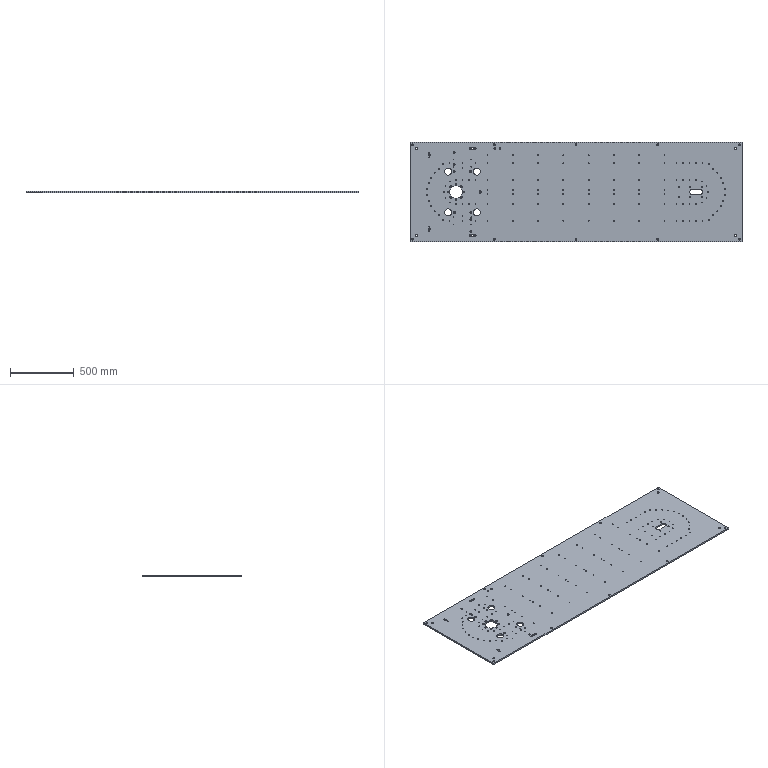Part | STEP file | Silo large plate | 1 solid | 465 faces | box 2600 x 780 x 12 mm | volume 23947596 mm3 | cylinder 431 | plane 34 | commonest cylinder face diameters 6.8 x240 9 x52 14 x52 5 x32 15 x24 8.5 x12